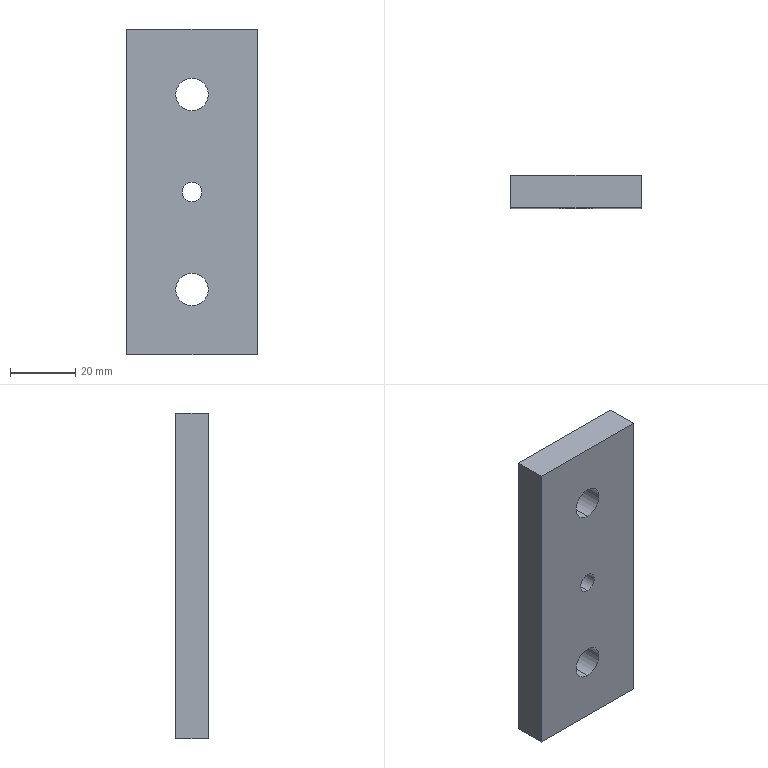Part | SolidWorks | features Extrusion 1 | 1 solid | 12 faces | box 40 x 10 x 100 mm | volume 38146 mm3 | cylinder 6 | plane 6 | commonest cylinder face diameters 10 x4 6 x2
STEP:
#1=CARTESIAN_POINT('',(0.,10.,-35.));
#2=VERTEX_POINT('',#1);
#3=CARTESIAN_POINT('',(0.,10.,-25.));
#4=VERTEX_POINT('',#3);
#5=CARTESIAN_POINT('',(0.,10.,-30.));
#6=DIRECTION('',(0.,1.,0.));
#7=DIRECTION('',(0.,0.,1.));
#8=AXIS2_PLACEMENT_3D('',#5,#6,#7);
#9=CIRCLE('',#8,5.);
#10=EDGE_CURVE('',#2,#4,#9,.T.);
#11=ORIENTED_EDGE('',*,*,#10,.T.);
#12=CARTESIAN_POINT('',(0.,0.,-25.));
#13=VERTEX_POINT('',#12);
#14=CARTESIAN_POINT('',(0.,10.,-25.));
#15=DIRECTION('',(0.,-1.,0.));
#16=VECTOR('',#15,1000.);
#17=LINE('',#14,#16);
#18=EDGE_CURVE('',#4,#13,#17,.T.);
#19=ORIENTED_EDGE('',*,*,#18,.T.);
#20=CARTESIAN_POINT('',(0.,0.,-35.));
#21=VERTEX_POINT('',#20);
#22=CARTESIAN_POINT('',(0.,0.,-30.));
#23=DIRECTION('',(0.,1.,0.));
#24=DIRECTION('',(0.,0.,1.));
#25=AXIS2_PLACEMENT_3D('',#22,#23,#24);
#26=CIRCLE('',#25,5.);
#27=EDGE_CURVE('',#21,#13,#26,.T.);
#28=ORIENTED_EDGE('',*,*,#27,.F.);
#29=CARTESIAN_POINT('',(0.,10.,-35.));
#30=DIRECTION('',(0.,-1.,0.));
#31=VECTOR('',#30,1000.);
#32=LINE('',#29,#31);
#33=EDGE_CURVE('',#2,#21,#32,.T.);
#34=ORIENTED_EDGE('',*,*,#33,.F.);
#35=EDGE_LOOP('',(#11,#19,#28,#34));
#36=FACE_OUTER_BOUND('',#35,.T.);
#37=CARTESIAN_POINT('',(0.,10.,-30.));
#38=DIRECTION('',(0.,-1.,0.));
#39=DIRECTION('',(0.,0.,-1.));
#40=AXIS2_PLACEMENT_3D('',#37,#38,#39);
#41=CYLINDRICAL_SURFACE('',#40,5.);
#42=ADVANCED_FACE('',(#36),#41,.F.);
#43=CARTESIAN_POINT('',(0.,10.,25.));
#44=VERTEX_POINT('',#43);
#45=CARTESIAN_POINT('',(0.,10.,35.));
#46=VERTEX_POINT('',#45);
#47=CARTESIAN_POINT('',(0.,10.,30.));
#48=DIRECTION('',(0.,1.,0.));
#49=DIRECTION('',(0.,0.,1.));
#50=AXIS2_PLACEMENT_3D('',#47,#48,#49);
#51=CIRCLE('',#50,5.);
#52=EDGE_CURVE('',#44,#46,#51,.T.);
#53=ORIENTED_EDGE('',*,*,#52,.T.);
#54=CARTESIAN_POINT('',(0.,0.,35.));
#55=VERTEX_POINT('',#54);
#56=CARTESIAN_POINT('',(0.,10.,35.));
#57=DIRECTION('',(0.,-1.,0.));
#58=VECTOR('',#57,1000.);
#59=LINE('',#56,#58);
#60=EDGE_CURVE('',#46,#55,#59,.T.);
#61=ORIENTED_EDGE('',*,*,#60,.T.);
#62=CARTESIAN_POINT('',(0.,0.,25.));
#63=VERTEX_POINT('',#62);
#64=CARTESIAN_POINT('',(0.,0.,30.));
#65=DIRECTION('',(0.,1.,0.));
#66=DIRECTION('',(0.,0.,1.));
#67=AXIS2_PLACEMENT_3D('',#64,#65,#66);
#68=CIRCLE('',#67,5.);
#69=EDGE_CURVE('',#63,#55,#68,.T.);
#70=ORIENTED_EDGE('',*,*,#69,.F.);
#71=CARTESIAN_POINT('',(0.,10.,25.));
#72=DIRECTION('',(0.,-1.,0.));
#73=VECTOR('',#72,1000.);
#74=LINE('',#71,#73);
#75=EDGE_CURVE('',#44,#63,#74,.T.);
#76=ORIENTED_EDGE('',*,*,#75,.F.);
#77=EDGE_LOOP('',(#53,#61,#70,#76));
#78=FACE_OUTER_BOUND('',#77,.T.);
#79=CARTESIAN_POINT('',(0.,10.,30.));
#80=DIRECTION('',(0.,-1.,0.));
#81=DIRECTION('',(0.,0.,-1.));
#82=AXIS2_PLACEMENT_3D('',#79,#80,#81);
#83=CYLINDRICAL_SURFACE('',#82,5.);
#84=ADVANCED_FACE('',(#78),#83,.F.);
#85=CARTESIAN_POINT('',(0.,10.,-3.));
#86=VERTEX_POINT('',#85);
#87=CARTESIAN_POINT('',(0.,10.,3.));
#88=VERTEX_POINT('',#87);
#89=CARTESIAN_POINT('',(0.,10.,0.));
#90=DIRECTION('',(0.,1.,0.));
#91=DIRECTION('',(0.,0.,1.));
#92=AXIS2_PLACEMENT_3D('',#89,#90,#91);
#93=CIRCLE('',#92,3.);
#94=EDGE_CURVE('',#86,#88,#93,.T.);
#95=ORIENTED_EDGE('',*,*,#94,.T.);
#96=CARTESIAN_POINT('',(0.,0.,3.));
#97=VERTEX_POINT('',#96);
#98=CARTESIAN_POINT('',(0.,10.,3.));
#99=DIRECTION('',(0.,-1.,0.));
#100=VECTOR('',#99,1000.);
#101=LINE('',#98,#100);
#102=EDGE_CURVE('',#88,#97,#101,.T.);
#103=ORIENTED_EDGE('',*,*,#102,.T.);
#104=CARTESIAN_POINT('',(0.,0.,-3.));
#105=VERTEX_POINT('',#104);
#106=CARTESIAN_POINT('',(0.,0.,0.));
#107=DIRECTION('',(0.,1.,0.));
#108=DIRECTION('',(0.,0.,1.));
#109=AXIS2_PLACEMENT_3D('',#106,#107,#108);
#110=CIRCLE('',#109,3.);
#111=EDGE_CURVE('',#105,#97,#110,.T.);
#112=ORIENTED_EDGE('',*,*,#111,.F.);
#113=CARTESIAN_POINT('',(0.,10.,-3.));
#114=DIRECTION('',(0.,-1.,0.));
#115=VECTOR('',#114,1000.);
#116=LINE('',#113,#115);
#117=EDGE_CURVE('',#86,#105,#116,.T.);
#118=ORIENTED_EDGE('',*,*,#117,.F.);
#119=EDGE_LOOP('',(#95,#103,#112,#118));
#120=FACE_OUTER_BOUND('',#119,.T.);
#121=CARTESIAN_POINT('',(0.,10.,0.));
#122=DIRECTION('',(0.,-1.,0.));
#123=DIRECTION('',(0.,0.,-1.));
#124=AXIS2_PLACEMENT_3D('',#121,#122,#123);
#125=CYLINDRICAL_SURFACE('',#124,3.);
#126=ADVANCED_FACE('',(#120),#125,.F.);
#127=CARTESIAN_POINT('',(20.,0.,-50.));
#128=VERTEX_POINT('',#127);
#129=CARTESIAN_POINT('',(-20.,0.,-50.));
#130=VERTEX_POINT('',#129);
#131=CARTESIAN_POINT('',(0.,0.,-50.));
#132=DIRECTION('',(-1.,0.,0.));
#133=VECTOR('',#132,1000.);
#134=LINE('',#131,#133);
#135=EDGE_CURVE('',#128,#130,#134,.T.);
#136=ORIENTED_EDGE('',*,*,#135,.T.);
#137=CARTESIAN_POINT('',(-20.,10.,-50.));
#138=VERTEX_POINT('',#137);
#139=CARTESIAN_POINT('',(-20.,10.,-50.));
#140=DIRECTION('',(0.,-1.,0.));
#141=VECTOR('',#140,1000.);
#142=LINE('',#139,#141);
#143=EDGE_CURVE('',#138,#130,#142,.T.);
#144=ORIENTED_EDGE('',*,*,#143,.F.);
#145=CARTESIAN_POINT('',(20.,10.,-50.));
#146=VERTEX_POINT('',#145);
#147=CARTESIAN_POINT('',(0.,10.,-50.));
#148=DIRECTION('',(-1.,0.,0.));
#149=VECTOR('',#148,1000.);
#150=LINE('',#147,#149);
#151=EDGE_CURVE('',#146,#138,#150,.T.);
#152=ORIENTED_EDGE('',*,*,#151,.F.);
#153=CARTESIAN_POINT('',(20.,10.,-50.));
#154=DIRECTION('',(0.,-1.,0.));
#155=VECTOR('',#154,1000.);
#156=LINE('',#153,#155);
#157=EDGE_CURVE('',#146,#128,#156,.T.);
#158=ORIENTED_EDGE('',*,*,#157,.T.);
#159=EDGE_LOOP('',(#136,#144,#152,#158));
#160=FACE_OUTER_BOUND('',#159,.T.);
#161=CARTESIAN_POINT('',(0.,10.,-50.));
#162=DIRECTION('',(0.,0.,1.));
#163=DIRECTION('',(1.,0.,0.));
#164=AXIS2_PLACEMENT_3D('',#161,#162,#163);
#165=PLANE('',#164);
#166=ADVANCED_FACE('',(#160),#165,.F.);
#167=CARTESIAN_POINT('',(-20.,0.,50.));
#168=VERTEX_POINT('',#167);
#169=CARTESIAN_POINT('',(-20.,0.,0.));
#170=DIRECTION('',(0.,0.,1.));
#171=VECTOR('',#170,1000.);
#172=LINE('',#169,#171);
#173=EDGE_CURVE('',#130,#168,#172,.T.);
#174=ORIENTED_EDGE('',*,*,#173,.T.);
#175=CARTESIAN_POINT('',(-20.,10.,50.));
#176=VERTEX_POINT('',#175);
#177=CARTESIAN_POINT('',(-20.,10.,50.));
#178=DIRECTION('',(0.,-1.,0.));
#179=VECTOR('',#178,1000.);
#180=LINE('',#177,#179);
#181=EDGE_CURVE('',#176,#168,#180,.T.);
#182=ORIENTED_EDGE('',*,*,#181,.F.);
#183=CARTESIAN_POINT('',(-20.,10.,0.));
#184=DIRECTION('',(0.,0.,1.));
#185=VECTOR('',#184,1000.);
#186=LINE('',#183,#185);
#187=EDGE_CURVE('',#138,#176,#186,.T.);
#188=ORIENTED_EDGE('',*,*,#187,.F.);
#189=ORIENTED_EDGE('',*,*,#143,.T.);
#190=EDGE_LOOP('',(#174,#182,#188,#189));
#191=FACE_OUTER_BOUND('',#190,.T.);
#192=CARTESIAN_POINT('',(-20.,10.,0.));
#193=DIRECTION('',(1.,0.,0.));
#194=DIRECTION('',(0.,0.,-1.));
#195=AXIS2_PLACEMENT_3D('',#192,#193,#194);
#196=PLANE('',#195);
#197=ADVANCED_FACE('',(#191),#196,.F.);
#198=CARTESIAN_POINT('',(20.,0.,50.));
#199=VERTEX_POINT('',#198);
#200=CARTESIAN_POINT('',(0.,0.,50.));
#201=DIRECTION('',(-1.,0.,0.));
#202=VECTOR('',#201,1000.);
#203=LINE('',#200,#202);
#204=EDGE_CURVE('',#199,#168,#203,.T.);
#205=ORIENTED_EDGE('',*,*,#204,.F.);
#206=CARTESIAN_POINT('',(20.,10.,50.));
#207=VERTEX_POINT('',#206);
#208=CARTESIAN_POINT('',(20.,10.,50.));
#209=DIRECTION('',(0.,-1.,0.));
#210=VECTOR('',#209,1000.);
#211=LINE('',#208,#210);
#212=EDGE_CURVE('',#207,#199,#211,.T.);
#213=ORIENTED_EDGE('',*,*,#212,.F.);
#214=CARTESIAN_POINT('',(0.,10.,50.));
#215=DIRECTION('',(-1.,0.,0.));
#216=VECTOR('',#215,1000.);
#217=LINE('',#214,#216);
#218=EDGE_CURVE('',#207,#176,#217,.T.);
#219=ORIENTED_EDGE('',*,*,#218,.T.);
#220=ORIENTED_EDGE('',*,*,#181,.T.);
#221=EDGE_LOOP('',(#205,#213,#219,#220));
#222=FACE_OUTER_BOUND('',#221,.T.);
#223=CARTESIAN_POINT('',(0.,10.,50.));
#224=DIRECTION('',(0.,0.,1.));
#225=DIRECTION('',(1.,0.,0.));
#226=AXIS2_PLACEMENT_3D('',#223,#224,#225);
#227=PLANE('',#226);
#228=ADVANCED_FACE('',(#222),#227,.T.);
#229=ORIENTED_EDGE('',*,*,#102,.F.);
#230=CARTESIAN_POINT('',(0.,10.,0.));
#231=DIRECTION('',(0.,1.,0.));
#232=DIRECTION('',(0.,0.,1.));
#233=AXIS2_PLACEMENT_3D('',#230,#231,#232);
#234=CIRCLE('',#233,3.);
#235=EDGE_CURVE('',#88,#86,#234,.T.);
#236=ORIENTED_EDGE('',*,*,#235,.T.);
#237=ORIENTED_EDGE('',*,*,#117,.T.);
#238=CARTESIAN_POINT('',(0.,0.,0.));
#239=DIRECTION('',(0.,1.,0.));
#240=DIRECTION('',(0.,0.,1.));
#241=AXIS2_PLACEMENT_3D('',#238,#239,#240);
#242=CIRCLE('',#241,3.);
#243=EDGE_CURVE('',#97,#105,#242,.T.);
#244=ORIENTED_EDGE('',*,*,#243,.F.);
#245=EDGE_LOOP('',(#229,#236,#237,#244));
#246=FACE_OUTER_BOUND('',#245,.T.);
#247=CARTESIAN_POINT('',(0.,10.,0.));
#248=DIRECTION('',(0.,-1.,0.));
#249=DIRECTION('',(0.,0.,-1.));
#250=AXIS2_PLACEMENT_3D('',#247,#248,#249);
#251=CYLINDRICAL_SURFACE('',#250,3.);
#252=ADVANCED_FACE('',(#246),#251,.F.);
#253=ORIENTED_EDGE('',*,*,#60,.F.);
#254=CARTESIAN_POINT('',(0.,10.,30.));
#255=DIRECTION('',(0.,1.,0.));
#256=DIRECTION('',(0.,0.,1.));
#257=AXIS2_PLACEMENT_3D('',#254,#255,#256);
#258=CIRCLE('',#257,5.);
#259=EDGE_CURVE('',#46,#44,#258,.T.);
#260=ORIENTED_EDGE('',*,*,#259,.T.);
#261=ORIENTED_EDGE('',*,*,#75,.T.);
#262=CARTESIAN_POINT('',(0.,0.,30.));
#263=DIRECTION('',(0.,1.,0.));
#264=DIRECTION('',(0.,0.,1.));
#265=AXIS2_PLACEMENT_3D('',#262,#263,#264);
#266=CIRCLE('',#265,5.);
#267=EDGE_CURVE('',#55,#63,#266,.T.);
#268=ORIENTED_EDGE('',*,*,#267,.F.);
#269=EDGE_LOOP('',(#253,#260,#261,#268));
#270=FACE_OUTER_BOUND('',#269,.T.);
#271=CARTESIAN_POINT('',(0.,10.,30.));
#272=DIRECTION('',(0.,-1.,0.));
#273=DIRECTION('',(0.,0.,-1.));
#274=AXIS2_PLACEMENT_3D('',#271,#272,#273);
#275=CYLINDRICAL_SURFACE('',#274,5.);
#276=ADVANCED_FACE('',(#270),#275,.F.);
#277=ORIENTED_EDGE('',*,*,#18,.F.);
#278=CARTESIAN_POINT('',(0.,10.,-30.));
#279=DIRECTION('',(0.,1.,0.));
#280=DIRECTION('',(0.,0.,1.));
#281=AXIS2_PLACEMENT_3D('',#278,#279,#280);
#282=CIRCLE('',#281,5.);
#283=EDGE_CURVE('',#4,#2,#282,.T.);
#284=ORIENTED_EDGE('',*,*,#283,.T.);
#285=ORIENTED_EDGE('',*,*,#33,.T.);
#286=CARTESIAN_POINT('',(0.,0.,-30.));
#287=DIRECTION('',(0.,1.,0.));
#288=DIRECTION('',(0.,0.,1.));
#289=AXIS2_PLACEMENT_3D('',#286,#287,#288);
#290=CIRCLE('',#289,5.);
#291=EDGE_CURVE('',#13,#21,#290,.T.);
#292=ORIENTED_EDGE('',*,*,#291,.F.);
#293=EDGE_LOOP('',(#277,#284,#285,#292));
#294=FACE_OUTER_BOUND('',#293,.T.);
#295=CARTESIAN_POINT('',(0.,10.,-30.));
#296=DIRECTION('',(0.,-1.,0.));
#297=DIRECTION('',(0.,0.,-1.));
#298=AXIS2_PLACEMENT_3D('',#295,#296,#297);
#299=CYLINDRICAL_SURFACE('',#298,5.);
#300=ADVANCED_FACE('',(#294),#299,.F.);
#301=CARTESIAN_POINT('',(20.,0.,0.));
#302=DIRECTION('',(0.,0.,1.));
#303=VECTOR('',#302,1000.);
#304=LINE('',#301,#303);
#305=EDGE_CURVE('',#128,#199,#304,.T.);
#306=ORIENTED_EDGE('',*,*,#305,.F.);
#307=ORIENTED_EDGE('',*,*,#157,.F.);
#308=CARTESIAN_POINT('',(20.,10.,0.));
#309=DIRECTION('',(0.,0.,1.));
#310=VECTOR('',#309,1000.);
#311=LINE('',#308,#310);
#312=EDGE_CURVE('',#146,#207,#311,.T.);
#313=ORIENTED_EDGE('',*,*,#312,.T.);
#314=ORIENTED_EDGE('',*,*,#212,.T.);
#315=EDGE_LOOP('',(#306,#307,#313,#314));
#316=FACE_OUTER_BOUND('',#315,.T.);
#317=CARTESIAN_POINT('',(20.,10.,0.));
#318=DIRECTION('',(1.,0.,0.));
#319=DIRECTION('',(0.,0.,-1.));
#320=AXIS2_PLACEMENT_3D('',#317,#318,#319);
#321=PLANE('',#320);
#322=ADVANCED_FACE('',(#316),#321,.T.);
#323=ORIENTED_EDGE('',*,*,#10,.F.);
#324=ORIENTED_EDGE('',*,*,#283,.F.);
#325=EDGE_LOOP('',(#323,#324));
#326=FACE_BOUND('',#325,.T.);
#327=ORIENTED_EDGE('',*,*,#52,.F.);
#328=ORIENTED_EDGE('',*,*,#259,.F.);
#329=EDGE_LOOP('',(#327,#328));
#330=FACE_BOUND('',#329,.T.);
#331=ORIENTED_EDGE('',*,*,#94,.F.);
#332=ORIENTED_EDGE('',*,*,#235,.F.);
#333=EDGE_LOOP('',(#331,#332));
#334=FACE_BOUND('',#333,.T.);
#335=ORIENTED_EDGE('',*,*,#151,.T.);
#336=ORIENTED_EDGE('',*,*,#187,.T.);
#337=ORIENTED_EDGE('',*,*,#218,.F.);
#338=ORIENTED_EDGE('',*,*,#312,.F.);
#339=EDGE_LOOP('',(#335,#336,#337,#338));
#340=FACE_OUTER_BOUND('',#339,.T.);
#341=CARTESIAN_POINT('',(0.,10.,0.));
#342=DIRECTION('',(0.,1.,0.));
#343=DIRECTION('',(0.,0.,1.));
#344=AXIS2_PLACEMENT_3D('',#341,#342,#343);
#345=PLANE('',#344);
#346=ADVANCED_FACE('',(#326,#330,#334,#340),#345,.T.);
#347=ORIENTED_EDGE('',*,*,#27,.T.);
#348=ORIENTED_EDGE('',*,*,#291,.T.);
#349=EDGE_LOOP('',(#347,#348));
#350=FACE_BOUND('',#349,.T.);
#351=ORIENTED_EDGE('',*,*,#69,.T.);
#352=ORIENTED_EDGE('',*,*,#267,.T.);
#353=EDGE_LOOP('',(#351,#352));
#354=FACE_BOUND('',#353,.T.);
#355=ORIENTED_EDGE('',*,*,#111,.T.);
#356=ORIENTED_EDGE('',*,*,#243,.T.);
#357=EDGE_LOOP('',(#355,#356));
#358=FACE_BOUND('',#357,.T.);
#359=ORIENTED_EDGE('',*,*,#135,.F.);
#360=ORIENTED_EDGE('',*,*,#305,.T.);
#361=ORIENTED_EDGE('',*,*,#204,.T.);
#362=ORIENTED_EDGE('',*,*,#173,.F.);
#363=EDGE_LOOP('',(#359,#360,#361,#362));
#364=FACE_OUTER_BOUND('',#363,.T.);
#365=CARTESIAN_POINT('',(0.,0.,0.));
#366=DIRECTION('',(0.,1.,0.));
#367=DIRECTION('',(0.,0.,1.));
#368=AXIS2_PLACEMENT_3D('',#365,#366,#367);
#369=PLANE('',#368);
#370=ADVANCED_FACE('',(#350,#354,#358,#364),#369,.F.);
#371=CLOSED_SHELL('',(#42,#84,#126,#166,#197,#228,#252,#276,#300,#322,#346,#370));
#372=MANIFOLD_SOLID_BREP('',#371);
#373=CARTESIAN_POINT('',(0.,0.,0.));
#374=DIRECTION('',(0.,0.,1.));
#375=DIRECTION('',(1.,0.,0.));
#376=AXIS2_PLACEMENT_3D('',#373,#374,#375);
#377=(LENGTH_UNIT()NAMED_UNIT(*)SI_UNIT(.MILLI.,.METRE.));
#378=UNCERTAINTY_MEASURE_WITH_UNIT(LENGTH_MEASURE(0.00001),#377,'','');
#379=(NAMED_UNIT(*)PLANE_ANGLE_UNIT()SI_UNIT($,.RADIAN.));
#380=(NAMED_UNIT(*)SI_UNIT($,.STERADIAN.)SOLID_ANGLE_UNIT());
#381=(GEOMETRIC_REPRESENTATION_CONTEXT(3)GLOBAL_UNCERTAINTY_ASSIGNED_CONTEXT((#378))GLOBAL_UNIT_ASSIGNED_CONTEXT((#377,#379,#380))REPRESENTATION_CONTEXT('',''));
#382=ADVANCED_BREP_SHAPE_REPRESENTATION('',(#372,#376),#381);